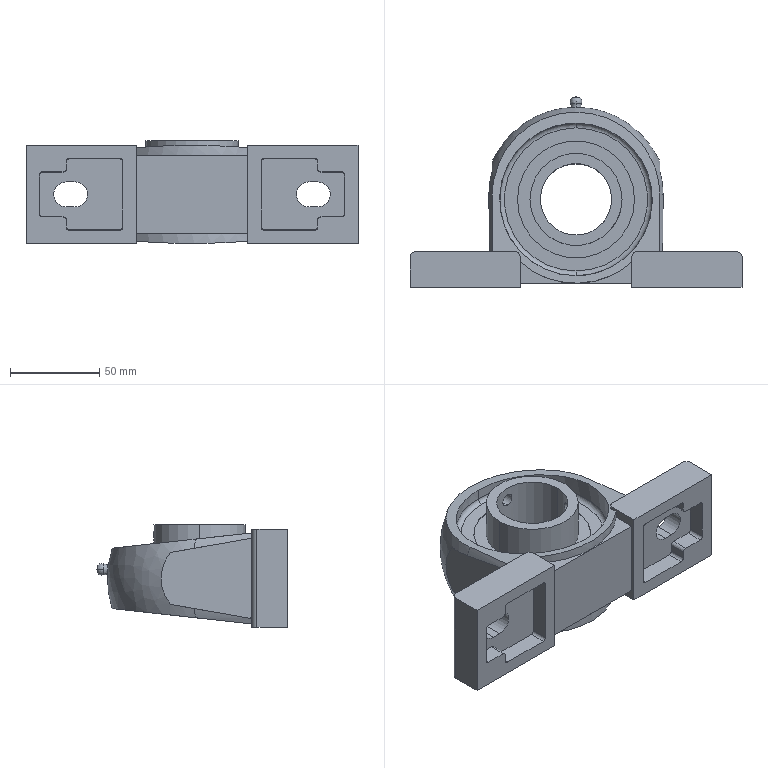Part | SolidWorks | features Revolution 5, Cut 3, Boss 2, CirPattern 2, ICE 2, RevCut 2, Extrusion 1, RefAxis 1, SweepCut 1 | 1 solid | 162 faces | box 186 x 106.8 x 57.7 mm | volume 279855 mm3 | plane 56 | cylinder 43 | sphere 34 | cone 16 | torus 8 | spline 5 | commonest cylinder face diameters 2 x6 6 x6 51.6 x6 65.64 x6 85.524 x6 7.134 x4